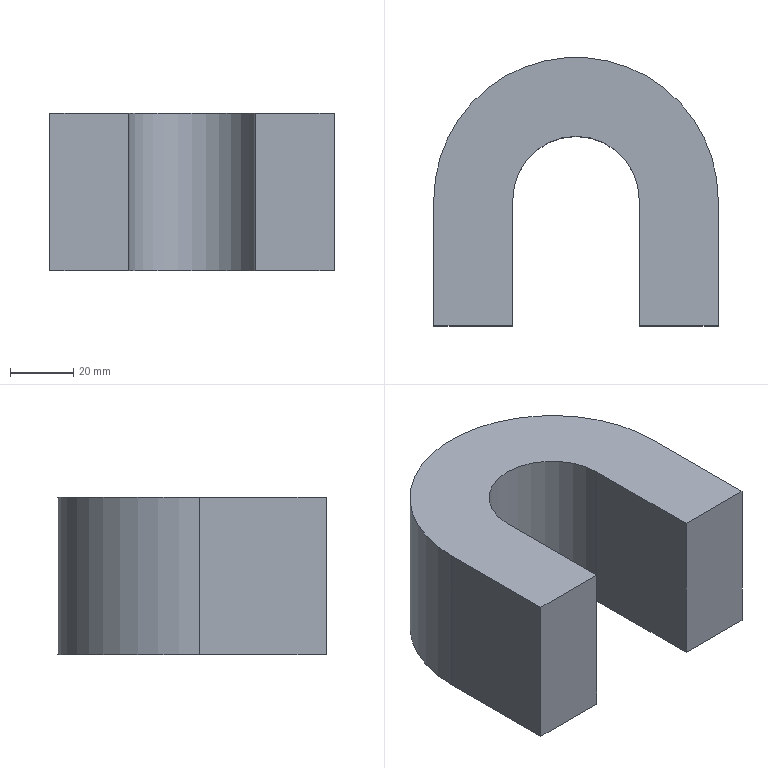Part | NX | features solid 2 | 1 solid | 10 faces | box 90 x 85 x 50 mm | volume 227627 mm3 | plane 8 | cylinder 2 | commonest cylinder face diameters 40 x1 90 x1
STEP:
#1=CARTESIAN_POINT('',(170.,-270.,-260.));
#2=VERTEX_POINT('',#1);
#3=CARTESIAN_POINT('',(170.,-310.,-260.));
#4=VERTEX_POINT('',#3);
#5=CARTESIAN_POINT('',(170.,-270.,-260.));
#6=DIRECTION('',(0.,-1.,0.));
#7=VECTOR('',#6,1000.);
#8=LINE('',#5,#7);
#9=EDGE_CURVE('',#2,#4,#8,.T.);
#10=ORIENTED_EDGE('',*,*,#9,.F.);
#11=CARTESIAN_POINT('',(170.,-270.,-310.));
#12=VERTEX_POINT('',#11);
#13=CARTESIAN_POINT('',(170.,-270.,-310.));
#14=DIRECTION('',(0.,0.,1.));
#15=VECTOR('',#14,1000.);
#16=LINE('',#13,#15);
#17=EDGE_CURVE('',#12,#2,#16,.T.);
#18=ORIENTED_EDGE('',*,*,#17,.F.);
#19=CARTESIAN_POINT('',(170.,-310.,-310.));
#20=VERTEX_POINT('',#19);
#21=CARTESIAN_POINT('',(170.,-270.,-310.));
#22=DIRECTION('',(0.,-1.,0.));
#23=VECTOR('',#22,1000.);
#24=LINE('',#21,#23);
#25=EDGE_CURVE('',#12,#20,#24,.T.);
#26=ORIENTED_EDGE('',*,*,#25,.T.);
#27=CARTESIAN_POINT('',(170.,-310.,-310.));
#28=DIRECTION('',(0.,0.,1.));
#29=VECTOR('',#28,1000.);
#30=LINE('',#27,#29);
#31=EDGE_CURVE('',#20,#4,#30,.T.);
#32=ORIENTED_EDGE('',*,*,#31,.T.);
#33=EDGE_LOOP('',(#10,#18,#26,#32));
#34=FACE_BOUND('',#33,.T.);
#35=CARTESIAN_POINT('',(170.,-270.,-310.));
#36=DIRECTION('',(-1.,0.,0.));
#37=DIRECTION('',(0.,0.,1.));
#38=AXIS2_PLACEMENT_3D('',#35,#36,#37);
#39=PLANE('',#38);
#40=ADVANCED_FACE('',(#34),#39,.T.);
#41=CARTESIAN_POINT('',(195.,-310.,-260.));
#42=VERTEX_POINT('',#41);
#43=CARTESIAN_POINT('',(-705.,-310.,-260.));
#44=DIRECTION('',(-1.,0.,0.));
#45=VECTOR('',#44,1000.);
#46=LINE('',#43,#45);
#47=EDGE_CURVE('',#42,#4,#46,.T.);
#48=ORIENTED_EDGE('',*,*,#47,.T.);
#49=ORIENTED_EDGE('',*,*,#31,.F.);
#50=CARTESIAN_POINT('',(195.,-310.,-310.));
#51=VERTEX_POINT('',#50);
#52=CARTESIAN_POINT('',(-705.,-310.,-310.));
#53=DIRECTION('',(-1.,0.,0.));
#54=VECTOR('',#53,1000.);
#55=LINE('',#52,#54);
#56=EDGE_CURVE('',#51,#20,#55,.T.);
#57=ORIENTED_EDGE('',*,*,#56,.F.);
#58=CARTESIAN_POINT('',(195.,-310.,-310.));
#59=DIRECTION('',(0.,0.,1.));
#60=VECTOR('',#59,1000.);
#61=LINE('',#58,#60);
#62=EDGE_CURVE('',#51,#42,#61,.T.);
#63=ORIENTED_EDGE('',*,*,#62,.T.);
#64=EDGE_LOOP('',(#48,#49,#57,#63));
#65=FACE_BOUND('',#64,.T.);
#66=CARTESIAN_POINT('',(-705.,-310.,-310.));
#67=DIRECTION('',(0.,1.,0.));
#68=DIRECTION('',(0.,0.,1.));
#69=AXIS2_PLACEMENT_3D('',#66,#67,#68);
#70=PLANE('',#69);
#71=ADVANCED_FACE('',(#65),#70,.F.);
#72=CARTESIAN_POINT('',(195.,-270.,-260.));
#73=VERTEX_POINT('',#72);
#74=CARTESIAN_POINT('',(195.,-270.,-260.));
#75=DIRECTION('',(0.,-1.,0.));
#76=VECTOR('',#75,1000.);
#77=LINE('',#74,#76);
#78=EDGE_CURVE('',#73,#42,#77,.T.);
#79=ORIENTED_EDGE('',*,*,#78,.T.);
#80=ORIENTED_EDGE('',*,*,#62,.F.);
#81=CARTESIAN_POINT('',(195.,-270.,-310.));
#82=VERTEX_POINT('',#81);
#83=CARTESIAN_POINT('',(195.,-270.,-310.));
#84=DIRECTION('',(0.,-1.,0.));
#85=VECTOR('',#84,1000.);
#86=LINE('',#83,#85);
#87=EDGE_CURVE('',#82,#51,#86,.T.);
#88=ORIENTED_EDGE('',*,*,#87,.F.);
#89=CARTESIAN_POINT('',(195.,-270.,-310.));
#90=DIRECTION('',(0.,0.,1.));
#91=VECTOR('',#90,1000.);
#92=LINE('',#89,#91);
#93=EDGE_CURVE('',#82,#73,#92,.T.);
#94=ORIENTED_EDGE('',*,*,#93,.T.);
#95=EDGE_LOOP('',(#79,#80,#88,#94));
#96=FACE_BOUND('',#95,.T.);
#97=CARTESIAN_POINT('',(195.,-270.,-310.));
#98=DIRECTION('',(-1.,0.,0.));
#99=DIRECTION('',(0.,0.,1.));
#100=AXIS2_PLACEMENT_3D('',#97,#98,#99);
#101=PLANE('',#100);
#102=ADVANCED_FACE('',(#96),#101,.F.);
#103=CARTESIAN_POINT('',(105.,-270.,-260.));
#104=VERTEX_POINT('',#103);
#105=CARTESIAN_POINT('',(150.,-270.,-260.));
#106=DIRECTION('',(0.,0.,1.));
#107=DIRECTION('',(1.,0.,0.));
#108=AXIS2_PLACEMENT_3D('',#105,#106,#107);
#109=CIRCLE('',#108,45.);
#110=EDGE_CURVE('',#104,#73,#109,.F.);
#111=ORIENTED_EDGE('',*,*,#110,.T.);
#112=ORIENTED_EDGE('',*,*,#93,.F.);
#113=CARTESIAN_POINT('',(105.,-270.,-310.));
#114=VERTEX_POINT('',#113);
#115=CARTESIAN_POINT('',(150.,-270.,-310.));
#116=DIRECTION('',(0.,0.,1.));
#117=DIRECTION('',(1.,0.,0.));
#118=AXIS2_PLACEMENT_3D('',#115,#116,#117);
#119=CIRCLE('',#118,45.);
#120=EDGE_CURVE('',#114,#82,#119,.F.);
#121=ORIENTED_EDGE('',*,*,#120,.F.);
#122=CARTESIAN_POINT('',(105.,-270.,-310.));
#123=DIRECTION('',(0.,0.,1.));
#124=VECTOR('',#123,1000.);
#125=LINE('',#122,#124);
#126=EDGE_CURVE('',#114,#104,#125,.T.);
#127=ORIENTED_EDGE('',*,*,#126,.T.);
#128=EDGE_LOOP('',(#111,#112,#121,#127));
#129=FACE_BOUND('',#128,.T.);
#130=CARTESIAN_POINT('',(150.,-270.,-310.));
#131=DIRECTION('',(0.,0.,1.));
#132=DIRECTION('',(1.,0.,0.));
#133=AXIS2_PLACEMENT_3D('',#130,#131,#132);
#134=CYLINDRICAL_SURFACE('',#133,45.);
#135=ADVANCED_FACE('',(#129),#134,.T.);
#136=CARTESIAN_POINT('',(105.,-310.,-260.));
#137=VERTEX_POINT('',#136);
#138=CARTESIAN_POINT('',(105.,-270.,-260.));
#139=DIRECTION('',(0.,-1.,0.));
#140=VECTOR('',#139,1000.);
#141=LINE('',#138,#140);
#142=EDGE_CURVE('',#104,#137,#141,.T.);
#143=ORIENTED_EDGE('',*,*,#142,.F.);
#144=ORIENTED_EDGE('',*,*,#126,.F.);
#145=CARTESIAN_POINT('',(105.,-310.,-310.));
#146=VERTEX_POINT('',#145);
#147=CARTESIAN_POINT('',(105.,-270.,-310.));
#148=DIRECTION('',(0.,-1.,0.));
#149=VECTOR('',#148,1000.);
#150=LINE('',#147,#149);
#151=EDGE_CURVE('',#114,#146,#150,.T.);
#152=ORIENTED_EDGE('',*,*,#151,.T.);
#153=CARTESIAN_POINT('',(105.,-310.,-310.));
#154=DIRECTION('',(0.,0.,1.));
#155=VECTOR('',#154,1000.);
#156=LINE('',#153,#155);
#157=EDGE_CURVE('',#146,#137,#156,.T.);
#158=ORIENTED_EDGE('',*,*,#157,.T.);
#159=EDGE_LOOP('',(#143,#144,#152,#158));
#160=FACE_BOUND('',#159,.T.);
#161=CARTESIAN_POINT('',(105.,-270.,-310.));
#162=DIRECTION('',(-1.,0.,0.));
#163=DIRECTION('',(0.,0.,1.));
#164=AXIS2_PLACEMENT_3D('',#161,#162,#163);
#165=PLANE('',#164);
#166=ADVANCED_FACE('',(#160),#165,.T.);
#167=CARTESIAN_POINT('',(130.,-310.,-260.));
#168=VERTEX_POINT('',#167);
#169=CARTESIAN_POINT('',(-705.,-310.,-260.));
#170=DIRECTION('',(-1.,0.,0.));
#171=VECTOR('',#170,1000.);
#172=LINE('',#169,#171);
#173=EDGE_CURVE('',#168,#137,#172,.T.);
#174=ORIENTED_EDGE('',*,*,#173,.T.);
#175=ORIENTED_EDGE('',*,*,#157,.F.);
#176=CARTESIAN_POINT('',(130.,-310.,-310.));
#177=VERTEX_POINT('',#176);
#178=CARTESIAN_POINT('',(-705.,-310.,-310.));
#179=DIRECTION('',(-1.,0.,0.));
#180=VECTOR('',#179,1000.);
#181=LINE('',#178,#180);
#182=EDGE_CURVE('',#177,#146,#181,.T.);
#183=ORIENTED_EDGE('',*,*,#182,.F.);
#184=CARTESIAN_POINT('',(130.,-310.,-310.));
#185=DIRECTION('',(0.,0.,1.));
#186=VECTOR('',#185,1000.);
#187=LINE('',#184,#186);
#188=EDGE_CURVE('',#177,#168,#187,.T.);
#189=ORIENTED_EDGE('',*,*,#188,.T.);
#190=EDGE_LOOP('',(#174,#175,#183,#189));
#191=FACE_BOUND('',#190,.T.);
#192=CARTESIAN_POINT('',(-705.,-310.,-310.));
#193=DIRECTION('',(0.,1.,0.));
#194=DIRECTION('',(0.,0.,1.));
#195=AXIS2_PLACEMENT_3D('',#192,#193,#194);
#196=PLANE('',#195);
#197=ADVANCED_FACE('',(#191),#196,.F.);
#198=CARTESIAN_POINT('',(130.,-270.,-260.));
#199=VERTEX_POINT('',#198);
#200=CARTESIAN_POINT('',(130.,-270.,-260.));
#201=DIRECTION('',(0.,-1.,0.));
#202=VECTOR('',#201,1000.);
#203=LINE('',#200,#202);
#204=EDGE_CURVE('',#199,#168,#203,.T.);
#205=ORIENTED_EDGE('',*,*,#204,.T.);
#206=ORIENTED_EDGE('',*,*,#188,.F.);
#207=CARTESIAN_POINT('',(130.,-270.,-310.));
#208=VERTEX_POINT('',#207);
#209=CARTESIAN_POINT('',(130.,-270.,-310.));
#210=DIRECTION('',(0.,-1.,0.));
#211=VECTOR('',#210,1000.);
#212=LINE('',#209,#211);
#213=EDGE_CURVE('',#208,#177,#212,.T.);
#214=ORIENTED_EDGE('',*,*,#213,.F.);
#215=CARTESIAN_POINT('',(130.,-270.,-310.));
#216=DIRECTION('',(0.,0.,1.));
#217=VECTOR('',#216,1000.);
#218=LINE('',#215,#217);
#219=EDGE_CURVE('',#208,#199,#218,.T.);
#220=ORIENTED_EDGE('',*,*,#219,.T.);
#221=EDGE_LOOP('',(#205,#206,#214,#220));
#222=FACE_BOUND('',#221,.T.);
#223=CARTESIAN_POINT('',(130.,-270.,-310.));
#224=DIRECTION('',(-1.,0.,0.));
#225=DIRECTION('',(0.,0.,1.));
#226=AXIS2_PLACEMENT_3D('',#223,#224,#225);
#227=PLANE('',#226);
#228=ADVANCED_FACE('',(#222),#227,.F.);
#229=CARTESIAN_POINT('',(150.,-270.,-260.));
#230=DIRECTION('',(0.,0.,1.));
#231=DIRECTION('',(1.,0.,0.));
#232=AXIS2_PLACEMENT_3D('',#229,#230,#231);
#233=CIRCLE('',#232,20.);
#234=EDGE_CURVE('',#199,#2,#233,.F.);
#235=ORIENTED_EDGE('',*,*,#234,.F.);
#236=ORIENTED_EDGE('',*,*,#219,.F.);
#237=CARTESIAN_POINT('',(150.,-270.,-310.));
#238=DIRECTION('',(0.,0.,1.));
#239=DIRECTION('',(1.,0.,0.));
#240=AXIS2_PLACEMENT_3D('',#237,#238,#239);
#241=CIRCLE('',#240,20.);
#242=EDGE_CURVE('',#208,#12,#241,.F.);
#243=ORIENTED_EDGE('',*,*,#242,.T.);
#244=ORIENTED_EDGE('',*,*,#17,.T.);
#245=EDGE_LOOP('',(#235,#236,#243,#244));
#246=FACE_BOUND('',#245,.T.);
#247=CARTESIAN_POINT('',(150.,-270.,-310.));
#248=DIRECTION('',(0.,0.,1.));
#249=DIRECTION('',(1.,0.,0.));
#250=AXIS2_PLACEMENT_3D('',#247,#248,#249);
#251=CYLINDRICAL_SURFACE('',#250,20.);
#252=ADVANCED_FACE('',(#246),#251,.F.);
#253=ORIENTED_EDGE('',*,*,#25,.F.);
#254=ORIENTED_EDGE('',*,*,#242,.F.);
#255=ORIENTED_EDGE('',*,*,#213,.T.);
#256=ORIENTED_EDGE('',*,*,#182,.T.);
#257=ORIENTED_EDGE('',*,*,#151,.F.);
#258=ORIENTED_EDGE('',*,*,#120,.T.);
#259=ORIENTED_EDGE('',*,*,#87,.T.);
#260=ORIENTED_EDGE('',*,*,#56,.T.);
#261=EDGE_LOOP('',(#253,#254,#255,#256,#257,#258,#259,#260));
#262=FACE_BOUND('',#261,.T.);
#263=CARTESIAN_POINT('',(150.,-270.,-310.));
#264=DIRECTION('',(0.,0.,1.));
#265=DIRECTION('',(1.,0.,0.));
#266=AXIS2_PLACEMENT_3D('',#263,#264,#265);
#267=PLANE('',#266);
#268=ADVANCED_FACE('',(#262),#267,.F.);
#269=ORIENTED_EDGE('',*,*,#9,.T.);
#270=ORIENTED_EDGE('',*,*,#47,.F.);
#271=ORIENTED_EDGE('',*,*,#78,.F.);
#272=ORIENTED_EDGE('',*,*,#110,.F.);
#273=ORIENTED_EDGE('',*,*,#142,.T.);
#274=ORIENTED_EDGE('',*,*,#173,.F.);
#275=ORIENTED_EDGE('',*,*,#204,.F.);
#276=ORIENTED_EDGE('',*,*,#234,.T.);
#277=EDGE_LOOP('',(#269,#270,#271,#272,#273,#274,#275,#276));
#278=FACE_BOUND('',#277,.T.);
#279=CARTESIAN_POINT('',(150.,-270.,-260.));
#280=DIRECTION('',(0.,0.,1.));
#281=DIRECTION('',(1.,0.,0.));
#282=AXIS2_PLACEMENT_3D('',#279,#280,#281);
#283=PLANE('',#282);
#284=ADVANCED_FACE('',(#278),#283,.T.);
#285=CLOSED_SHELL('',(#40,#71,#102,#135,#166,#197,#228,#252,#268,#284));
#286=MANIFOLD_SOLID_BREP('',#285);
#287=(LENGTH_UNIT()NAMED_UNIT(*)SI_UNIT(.MILLI.,.METRE.));
#288=UNCERTAINTY_MEASURE_WITH_UNIT(LENGTH_MEASURE(0.00001),#287,'','');
#289=(NAMED_UNIT(*)PLANE_ANGLE_UNIT()SI_UNIT($,.RADIAN.));
#290=(NAMED_UNIT(*)SI_UNIT($,.STERADIAN.)SOLID_ANGLE_UNIT());
#291=(GEOMETRIC_REPRESENTATION_CONTEXT(3)GLOBAL_UNCERTAINTY_ASSIGNED_CONTEXT((#288))GLOBAL_UNIT_ASSIGNED_CONTEXT((#287,#289,#290))REPRESENTATION_CONTEXT('',''));
#292=ADVANCED_BREP_SHAPE_REPRESENTATION('',(#286),#291);